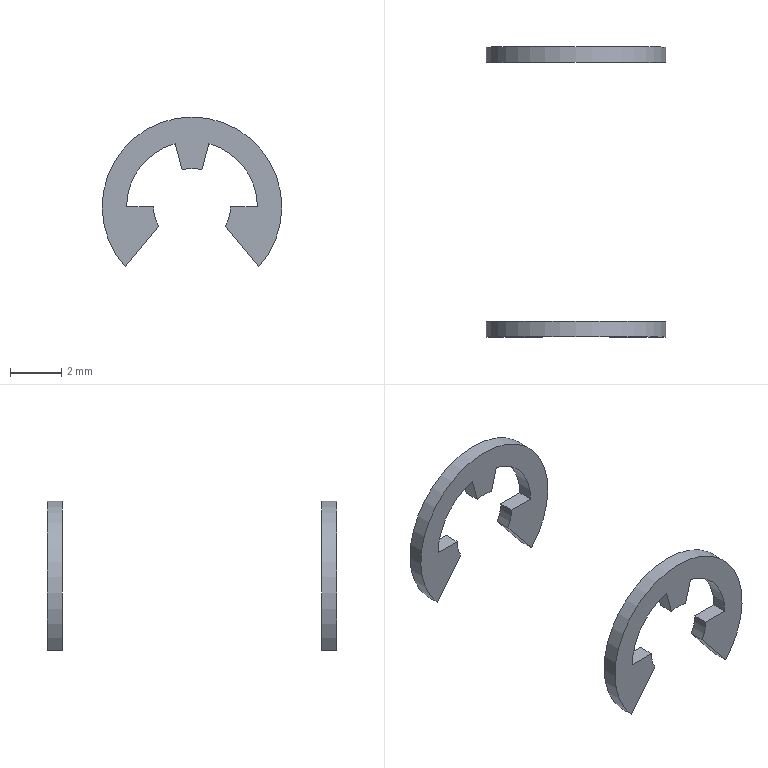Part | NX | 2 solids | 28 faces | box 7 x 11.3 x 5.843 mm | volume 20.221 mm3 | plane 16 | cylinder 12 | commonest cylinder face diameters 3 x6 5.1 x4 7 x2